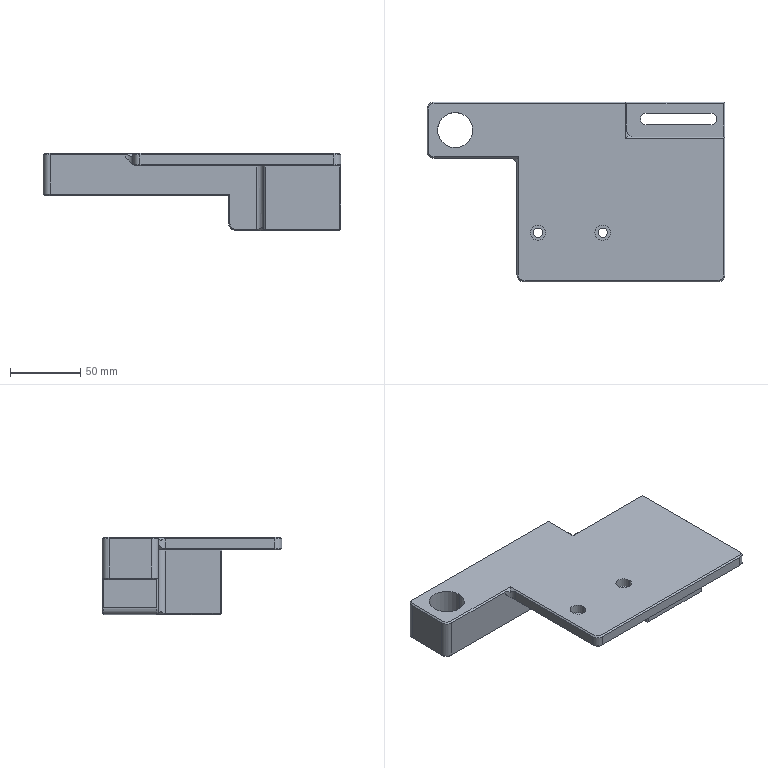NC program | NX | posted with a generic post | part box 212 x 128 x 55 mm
Lines 2820 to 4577 of 8014, first 1515 of 1754 lines:
(ZLEVEL_PROFILE_COPY_COPY_COPY_COPY , TOOL : D17R0.8)
N5632 T19 M6
N5634 G54
N5636 G17 G0 G90 X-28.227 Y13.355 S2000 M3
N5638 G43 Z30. H19
N5640 Z-0.3
N5642 G94 G1 X-29.568 Y15.677 F1000.
N5644 G3 X-31.04 Y16.527 R1.7
N5646 G1 X-43.527 F2000.
N5648 Y3.063
N5650 G3 X-42.677 Y1.59 R1.7
N5652 G1 X-40.127 Y0.118
N5654 G0 X-26.374 Y13.496 Z-0.6
N5656 G1 X-27.97 Y15.643 F1000.
N5658 G3 X-29.53 Y16.318 R1.7
N5660 G2 X-31. Y16.227 R13.652 F2000.
N5662 G1 X-43.227
N5664 Y0.892
N5666 G3 X-42.377 Y-0.58 R1.7
N5668 G1 X-39.827 Y-2.053
N5670 G0 X-26.137 Y13.28 Z-0.9
N5672 G1 X-27.774 Y15.404 F1000.
N5674 G3 X-29.346 Y16.05 R1.7
N5676 G2 X-31. Y15.927 R14.084 F2000.
N5678 G1 X-42.927
N5680 Y0.64
N5682 G3 X-42.077 Y-0.832 R1.7
N5684 G1 X-39.527 Y-2.304
N5686 G0 X-26.071 Y13.026 Z-1.2
N5688 G1 X-27.73 Y15.138 F1000.
N5690 G3 X-29.308 Y15.771 R1.7
N5692 G2 X-31.012 Y15.629 R14.424 F2000.
N5694 G1 X-42.629
N5696 Y0.569
N5698 G3 X-41.779 Y-0.904 R1.7
N5700 G1 X-39.229 Y-2.376
N5702 G0 X-26.037 Y12.748 Z-1.5
N5704 G1 X-27.588 Y14.865 F1000.
N5706 G3 X-29.144 Y15.549 R1.7
N5708 G2 X-30.099 Y15.488 R10.701 F2000.
N5710 G1 X-30.957 Y15.471
N5712 X-31.011 Y15.451
N5714 X-42.451
N5716 Y1.17
N5718 G3 X-41.601 Y-0.302 R1.7
N5720 G1 X-39.051 Y-1.774
N5722 G0 X-26.066 Y12.553 Z-1.8
N5724 G1 X-27.579 Y14.73 F1000.
N5726 G3 X-29.117 Y15.455 R1.7
N5728 G2 X-30.422 Y15.4 R15.644 F2000.
N5730 G1 X-42.4
N5732 Y1.03
N5734 G3 X-41.55 Y-0.442 R1.7
N5736 G1 X-39. Y-1.914
N5738 G0 X-25.877 Y12.452 Z-2.1
N5740 G1 X-27.297 Y14.641 F1000.
N5742 G3 X-28.811 Y15.413 R1.7
N5744 G2 X-29.33 Y15.4 R10.016 F2000.
N5746 G1 X-42.4
N5748 Y0.104
N5750 G3 X-41.55 Y-1.369 R1.7
N5752 G1 X-39. Y-2.841
N5754 G0 X-25.403 Y12.466 Z-2.4
N5756 G1 X-26.824 Y14.645 F1000.
N5758 G3 X-28.34 Y15.414 R1.7
N5760 G2 X-28.864 Y15.4 R9.678 F2000.
N5762 G1 X-42.4
N5764 Y0.011
N5766 G3 X-41.55 Y-1.461 R1.7
N5768 G1 X-39. Y-2.933
N5770 G0 X-25.124 Y12.447 Z-2.7
N5772 G1 X-26.527 Y14.632 F1000.
N5774 G3 X-28.038 Y15.411 R1.7
N5776 G2 X-28.475 Y15.4 R9.485 F2000.
N5778 G1 X-42.4
N5780 Y-0.04
N5782 G3 X-41.55 Y-1.512 R1.7
N5784 G1 X-39. Y-2.985
N5786 G0 X-24.937 Y12.419 Z-3.
N5788 G1 X-26.31 Y14.61 F1000.
N5790 G3 X-27.812 Y15.406 R1.7
N5792 G2 X-28.141 Y15.4 R9.072 F2000.
N5794 G1 X-42.4
N5796 Y-0.075
N5798 G3 X-41.55 Y-1.547 R1.7
N5800 G1 X-39. Y-3.019
N5802 G0 X-24.822 Y12.385 Z-3.3
N5804 G1 X-26.168 Y14.589 F1000.
N5806 G3 X-27.661 Y15.403 R1.7
N5808 G2 X-27.879 Y15.4 R8.949 F2000.
N5810 G1 X-42.4
N5812 Y-0.097
N5814 G3 X-41.55 Y-1.569 R1.7
N5816 G1 X-39. Y-3.041
N5818 G0 X-24.674 Y12.375 Z-3.6
N5820 G1 X-26.013 Y14.584 F1000.
N5822 G3 X-27.503 Y15.402 R1.7
N5824 G1 X-27.659 Y15.4 F2000.
N5826 X-42.4
N5828 Y-0.118
N5830 G3 X-41.55 Y-1.59 R1.7
N5832 G1 X-39. Y-3.062
N5834 G0 X-24.633 Y12.336 Z-3.9
N5836 G1 X-25.932 Y14.558 F1000.
N5838 G3 X-27.409 Y15.4 R1.7
N5840 G1 X-42.4 F2000.
N5842 Y-0.129
N5844 G3 X-41.55 Y-1.602 R1.7
N5846 G1 X-39. Y-3.074
N5848 G0 X-24.54 Y12.332 Z-4.2
N5850 G1 X-25.84 Y14.558 F1000.
N5852 G3 X-27.317 Y15.4 R1.7
N5854 G1 X-42.4 F2000.
N5856 Y-0.14
N5858 G3 X-41.55 Y-1.613 R1.7
N5860 G1 X-39. Y-3.085
N5862 G0 X-24.409 Y12.34 Z-4.5
N5864 G1 X-25.715 Y14.562 F1000.
N5866 G3 X-27.194 Y15.4 R1.7
N5868 G1 X-42.4 F2000.
N5870 Y-0.154
N5872 G3 X-41.55 Y-1.626 R1.7
N5874 G1 X-39. Y-3.099
N5876 G0 X-24.384 Y12.327 Z-4.8
N5878 G1 X-25.682 Y14.556 F1000.
N5880 G3 X-27.158 Y15.4 R1.7
N5882 G1 X-42.4 F2000.
N5884 Y-0.158
N5886 G3 X-41.55 Y-1.63 R1.7
N5888 G1 X-39. Y-3.103
N5890 G0 X-24.358 Y12.311 Z-5.1
N5892 G1 X-25.651 Y14.55 F1000.
N5894 G3 X-27.123 Y15.4 R1.7
N5896 G1 X-42.4 F2000.
N5898 Y-0.162
N5900 G3 X-41.55 Y-1.634 R1.7
N5902 G1 X-39. Y-3.106
N5904 G0 X-24.286 Y12.317 Z-5.4
N5906 G1 X-25.576 Y14.55 F1000.
N5908 G3 X-27.048 Y15.4 R1.7
N5910 G1 X-42.4 F2000.
N5912 Y-0.192
N5914 G3 X-41.55 Y-1.664 R1.7
N5916 G1 X-39. Y-3.136
N5918 G0 X-24.272 Y12.315 Z-5.7
N5920 G1 X-25.563 Y14.55 F1000.
N5922 G3 X-27.035 Y15.4 R1.7
N5924 G1 X-42.4 F2000.
N5926 Y-0.192
N5928 G3 X-41.55 Y-1.664 R1.7
N5930 G1 X-39. Y-3.136
N5932 G0 X-24.3 Y12.308 Z-6.
N5934 G1 X-25.595 Y14.55 F1000.
N5936 G3 X-27.067 Y15.4 R1.7
N5938 G1 X-42.4 F2000.
N5940 Y-0.167
N5942 G3 X-41.55 Y-1.64 R1.7
N5944 G1 X-39. Y-3.112
N5946 G0 X-24.3 Y12.308 Z-6.3
N5948 G1 X-25.595 Y14.55 F1000.
N5950 G3 X-27.067 Y15.4 R1.7
N5952 G1 X-42.4 F2000.
N5954 Y-0.167
N5956 G3 X-41.55 Y-1.64 R1.7
N5958 G1 X-39. Y-3.112
N5960 G0 X-24.3 Y12.308 Z-6.6
N5962 G1 X-25.595 Y14.55 F1000.
N5964 G3 X-27.067 Y15.4 R1.7
N5966 G1 X-42.4 F2000.
N5968 Y-0.167
N5970 G3 X-41.55 Y-1.64 R1.7
N5972 G1 X-39. Y-3.112
N5974 G0 X-24.3 Y12.308 Z-6.9
N5976 G1 X-25.595 Y14.55 F1000.
N5978 G3 X-27.067 Y15.4 R1.7
N5980 G1 X-42.4 F2000.
N5982 Y-0.167
N5984 G3 X-41.55 Y-1.64 R1.7
N5986 G1 X-39. Y-3.112
N5988 G0 X-24.3 Y12.308 Z-7.2
N5990 G1 X-25.595 Y14.55 F1000.
N5992 G3 X-27.067 Y15.4 R1.7
N5994 G1 X-42.4 F2000.
N5996 Y-0.167
N5998 G3 X-41.55 Y-1.64 R1.7
N6000 G1 X-39. Y-3.112
N6002 G0 X-24.3 Y12.308 Z-7.5
N6004 G1 X-25.595 Y14.55 F1000.
N6006 G3 X-27.067 Y15.4 R1.7
N6008 G1 X-42.4 F2000.
N6010 Y-0.167
N6012 G3 X-41.55 Y-1.64 R1.7
N6014 G1 X-39. Y-3.112
N6016 G0 X-24.3 Y12.308 Z-7.8
N6018 G1 X-25.595 Y14.55 F1000.
N6020 G3 X-27.067 Y15.4 R1.7
N6022 G1 X-42.4 F2000.
N6024 Y-0.167
N6026 G3 X-41.55 Y-1.64 R1.7
N6028 G1 X-39. Y-3.112
N6030 G0 X-24.3 Y12.308 Z-8.1
N6032 G1 X-25.595 Y14.55 F1000.
N6034 G3 X-27.067 Y15.4 R1.7
N6036 G1 X-42.4 F2000.
N6038 Y-0.167
N6040 G3 X-41.55 Y-1.64 R1.7
N6042 G1 X-39. Y-3.112
N6044 G0 X-24.3 Y12.308 Z-8.4
N6046 G1 X-25.595 Y14.55 F1000.
N6048 G3 X-27.067 Y15.4 R1.7
N6050 G1 X-42.4 F2000.
N6052 Y-0.167
N6054 G3 X-41.55 Y-1.64 R1.7
N6056 G1 X-39. Y-3.112
N6058 G0 X-24.3 Y12.308 Z-8.7
N6060 G1 X-25.595 Y14.55 F1000.
N6062 G3 X-27.067 Y15.4 R1.7
N6064 G1 X-42.4 F2000.
N6066 Y-0.167
N6068 G3 X-41.55 Y-1.64 R1.7
N6070 G1 X-39. Y-3.112
N6072 G0 X-24.3 Y12.308 Z-9.
N6074 G1 X-25.595 Y14.55 F1000.
N6076 G3 X-27.067 Y15.4 R1.7
N6078 G1 X-42.4 F2000.
N6080 Y-0.167
N6082 G3 X-41.55 Y-1.64 R1.7
N6084 G1 X-39. Y-3.112
N6086 G0 X-24.3 Y12.308 Z-9.3
N6088 G1 X-25.595 Y14.55 F1000.
N6090 G3 X-27.067 Y15.4 R1.7
N6092 G1 X-42.4 F2000.
N6094 Y-0.167
N6096 G3 X-41.55 Y-1.64 R1.7
N6098 G1 X-39. Y-3.112
N6100 G0 X-24.3 Y12.308 Z-9.6
N6102 G1 X-25.595 Y14.55 F1000.
N6104 G3 X-27.067 Y15.4 R1.7
N6106 G1 X-42.4 F2000.
N6108 Y-0.167
N6110 G3 X-41.55 Y-1.64 R1.7
N6112 G1 X-39. Y-3.112
N6114 G0 X-24.3 Y12.308 Z-9.9
N6116 G1 X-25.595 Y14.55 F1000.
N6118 G3 X-27.067 Y15.4 R1.7
N6120 G1 X-42.4 F2000.
N6122 Y-0.167
N6124 G3 X-41.55 Y-1.64 R1.7
N6126 G1 X-39. Y-3.112
N6128 G0 X-24.3 Y12.308 Z-10.2
N6130 G1 X-25.595 Y14.55 F1000.
N6132 G3 X-27.067 Y15.4 R1.7
N6134 G1 X-42.4 F2000.
N6136 Y-0.167
N6138 G3 X-41.55 Y-1.64 R1.7
N6140 G1 X-39. Y-3.112
N6142 G0 X-24.3 Y12.308 Z-10.5
N6144 G1 X-25.595 Y14.55 F1000.
N6146 G3 X-27.067 Y15.4 R1.7
N6148 G1 X-42.4 F2000.
N6150 Y-0.167
N6152 G3 X-41.55 Y-1.64 R1.7
N6154 G1 X-39. Y-3.112
N6156 G0 X-24.3 Y12.308 Z-10.8
N6158 G1 X-25.595 Y14.55 F1000.
N6160 G3 X-27.067 Y15.4 R1.7
N6162 G1 X-42.4 F2000.
N6164 Y-0.167
N6166 G3 X-41.55 Y-1.64 R1.7
N6168 G1 X-39. Y-3.112
N6170 G0 X-24.3 Y12.308 Z-11.1
N6172 G1 X-25.595 Y14.55 F1000.
N6174 G3 X-27.067 Y15.4 R1.7
N6176 G1 X-42.4 F2000.
N6178 Y-0.167
N6180 G3 X-41.55 Y-1.64 R1.7
N6182 G1 X-39. Y-3.112
N6184 G0 X-24.3 Y12.308 Z-11.4
N6186 G1 X-25.595 Y14.55 F1000.
N6188 G3 X-27.067 Y15.4 R1.7
N6190 G1 X-42.4 F2000.
N6192 Y-0.167
N6194 G3 X-41.55 Y-1.64 R1.7
N6196 G1 X-39. Y-3.112
N6198 G0 X-24.3 Y12.308 Z-11.7
N6200 G1 X-25.595 Y14.55 F1000.
N6202 G3 X-27.067 Y15.4 R1.7
N6204 G1 X-42.4 F2000.
N6206 Y-0.167
N6208 G3 X-41.55 Y-1.64 R1.7
N6210 G1 X-39. Y-3.112
N6212 G0 X-24.3 Y12.308 Z-12.
N6214 G1 X-25.595 Y14.55 F1000.
N6216 G3 X-27.067 Y15.4 R1.7
N6218 G1 X-42.4 F2000.
N6220 Y-0.167
N6222 G3 X-41.55 Y-1.64 R1.7
N6224 G1 X-39. Y-3.112
N6226 G0 X-24.3 Y12.308 Z-12.3
N6228 G1 X-25.595 Y14.55 F1000.
N6230 G3 X-27.067 Y15.4 R1.7
N6232 G1 X-42.4 F2000.
N6234 Y-0.167
N6236 G3 X-41.55 Y-1.64 R1.7
N6238 G1 X-39. Y-3.112
N6240 G0 X-24.3 Y12.308 Z-12.6
N6242 G1 X-25.595 Y14.55 F1000.
N6244 G3 X-27.067 Y15.4 R1.7
N6246 G1 X-42.4 F2000.
N6248 Y-0.167
N6250 G3 X-41.55 Y-1.64 R1.7
N6252 G1 X-39. Y-3.112
N6254 G0 X-24.3 Y12.308 Z-12.9
N6256 G1 X-25.595 Y14.55 F1000.
N6258 G3 X-27.067 Y15.4 R1.7
N6260 G1 X-42.4 F2000.
N6262 Y-0.167
N6264 G3 X-41.55 Y-1.64 R1.7
N6266 G1 X-39. Y-3.112
N6268 G0 X-24.3 Y12.308 Z-13.2
N6270 G1 X-25.595 Y14.55 F1000.
N6272 G3 X-27.067 Y15.4 R1.7
N6274 G1 X-42.4 F2000.
N6276 Y-0.167
N6278 G3 X-41.55 Y-1.64 R1.7
N6280 G1 X-39. Y-3.112
N6282 G0 X-24.3 Y12.308 Z-13.5
N6284 G1 X-25.595 Y14.55 F1000.
N6286 G3 X-27.067 Y15.4 R1.7
N6288 G1 X-42.4 F2000.
N6290 Y-0.167
N6292 G3 X-41.55 Y-1.64 R1.7
N6294 G1 X-39. Y-3.112
N6296 G0 X-24.3 Y12.308 Z-13.8
N6298 G1 X-25.595 Y14.55 F1000.
N6300 G3 X-27.067 Y15.4 R1.7
N6302 G1 X-42.4 F2000.
N6304 Y-0.167
N6306 G3 X-41.55 Y-1.64 R1.7
N6308 G1 X-39. Y-3.112
N6310 G0 X-24.3 Y12.308 Z-14.1
N6312 G1 X-25.595 Y14.55 F1000.
N6314 G3 X-27.067 Y15.4 R1.7
N6316 G1 X-42.4 F2000.
N6318 Y-0.167
N6320 G3 X-41.55 Y-1.64 R1.7
N6322 G1 X-39. Y-3.112
N6324 G0 X-24.3 Y12.308 Z-14.4
N6326 G1 X-25.595 Y14.55 F1000.
N6328 G3 X-27.067 Y15.4 R1.7
N6330 G1 X-42.4 F2000.
N6332 Y-0.167
N6334 G3 X-41.55 Y-1.64 R1.7
N6336 G1 X-39. Y-3.112
N6338 G0 X-24.3 Y12.308 Z-14.7
N6340 G1 X-25.595 Y14.55 F1000.
N6342 G3 X-27.067 Y15.4 R1.7
N6344 G1 X-42.4 F2000.
N6346 Y-0.167
N6348 G3 X-41.55 Y-1.64 R1.7
N6350 G1 X-39. Y-3.112
N6352 G0 X-24.3 Y12.308 Z-15.
N6354 G1 X-25.595 Y14.55 F1000.
N6356 G3 X-27.067 Y15.4 R1.7
N6358 G1 X-42.4 F2000.
N6360 Y-0.167
N6362 G3 X-41.55 Y-1.64 R1.7
N6364 G1 X-39. Y-3.112
N6366 G0 X-24.3 Y12.308 Z-15.3
N6368 G1 X-25.595 Y14.55 F1000.
N6370 G3 X-27.067 Y15.4 R1.7
N6372 G1 X-42.4 F2000.
N6374 Y-0.167
N6376 G3 X-41.55 Y-1.64 R1.7
N6378 G1 X-39. Y-3.112
N6380 G0 X-24.3 Y12.308 Z-15.6
N6382 G1 X-25.595 Y14.55 F1000.
N6384 G3 X-27.067 Y15.4 R1.7
N6386 G1 X-42.4 F2000.
N6388 Y-0.167
N6390 G3 X-41.55 Y-1.64 R1.7
N6392 G1 X-39. Y-3.112
N6394 G0 X-24.3 Y12.308 Z-15.9
N6396 G1 X-25.595 Y14.55 F1000.
N6398 G3 X-27.067 Y15.4 R1.7
N6400 G1 X-42.4 F2000.
N6402 Y-0.167
N6404 G3 X-41.55 Y-1.64 R1.7
N6406 G1 X-39. Y-3.112
N6408 G0 X-24.3 Y12.308 Z-16.2
N6410 G1 X-25.595 Y14.55 F1000.
N6412 G3 X-27.067 Y15.4 R1.7
N6414 G1 X-42.4 F2000.
N6416 Y-0.167
N6418 G3 X-41.55 Y-1.64 R1.7
N6420 G1 X-39. Y-3.112
N6422 G0 X-24.3 Y12.308 Z-16.5
N6424 G1 X-25.595 Y14.55 F1000.
N6426 G3 X-27.067 Y15.4 R1.7
N6428 G1 X-42.4 F2000.
N6430 Y-0.167
N6432 G3 X-41.55 Y-1.64 R1.7
N6434 G1 X-39. Y-3.112
N6436 G0 X-24.3 Y12.308 Z-16.8
N6438 G1 X-25.595 Y14.55 F1000.
N6440 G3 X-27.067 Y15.4 R1.7
N6442 G1 X-42.4 F2000.
N6444 Y-0.167
N6446 G3 X-41.55 Y-1.64 R1.7
N6448 G1 X-39. Y-3.112
N6450 G0 X-24.3 Y12.308 Z-17.1
N6452 G1 X-25.595 Y14.55 F1000.
N6454 G3 X-27.067 Y15.4 R1.7
N6456 G1 X-42.4 F2000.
N6458 Y-0.167
N6460 G3 X-41.55 Y-1.64 R1.7
N6462 G1 X-39. Y-3.112
N6464 G0 X-24.3 Y12.308 Z-17.4
N6466 G1 X-25.595 Y14.55 F1000.
N6468 G3 X-27.067 Y15.4 R1.7
N6470 G1 X-42.4 F2000.
N6472 Y-0.167
N6474 G3 X-41.55 Y-1.64 R1.7
N6476 G1 X-39. Y-3.112
N6478 G0 X-24.3 Y12.308 Z-17.7
N6480 G1 X-25.595 Y14.55 F1000.
N6482 G3 X-27.067 Y15.4 R1.7
N6484 G1 X-42.4 F2000.
N6486 Y-0.167
N6488 G3 X-41.55 Y-1.64 R1.7
N6490 G1 X-39. Y-3.112
N6492 G0 X-24.3 Y12.308 Z-18.
N6494 G1 X-25.595 Y14.55 F1000.
N6496 G3 X-27.067 Y15.4 R1.7
N6498 G1 X-42.4 F2000.
N6500 Y-0.167
N6502 G3 X-41.55 Y-1.64 R1.7
N6504 G1 X-39. Y-3.112
N6506 G0 X-24.3 Y12.308 Z-18.3
N6508 G1 X-25.595 Y14.55 F1000.
N6510 G3 X-27.067 Y15.4 R1.7
N6512 G1 X-42.4 F2000.
N6514 Y-0.167
N6516 G3 X-41.55 Y-1.64 R1.7
N6518 G1 X-39. Y-3.112
N6520 G0 X-24.3 Y12.308 Z-18.6
N6522 G1 X-25.595 Y14.55 F1000.
N6524 G3 X-27.067 Y15.4 R1.7
N6526 G1 X-42.4 F2000.
N6528 Y-0.167
N6530 G3 X-41.55 Y-1.64 R1.7
N6532 G1 X-39. Y-3.112
N6534 G0 X-24.3 Y12.308 Z-18.9
N6536 G1 X-25.595 Y14.55 F1000.
N6538 G3 X-27.067 Y15.4 R1.7
N6540 G1 X-42.4 F2000.
N6542 Y-0.167
N6544 G3 X-41.55 Y-1.64 R1.7
N6546 G1 X-39. Y-3.112
N6548 G0 X-24.3 Y12.308 Z-19.2
N6550 G1 X-25.595 Y14.55 F1000.
N6552 G3 X-27.067 Y15.4 R1.7
N6554 G1 X-42.4 F2000.
N6556 Y-0.167
N6558 G3 X-41.55 Y-1.64 R1.7
N6560 G1 X-39. Y-3.112
N6562 G0 X-24.3 Y12.308 Z-19.5
N6564 G1 X-25.595 Y14.55 F1000.
N6566 G3 X-27.067 Y15.4 R1.7
N6568 G1 X-42.4 F2000.
N6570 Y-0.167
N6572 G3 X-41.55 Y-1.64 R1.7
N6574 G1 X-39. Y-3.112
N6576 G0 X-24.3 Y12.308 Z-19.8
N6578 G1 X-25.595 Y14.55 F1000.
N6580 G3 X-27.067 Y15.4 R1.7
N6582 G1 X-42.4 F2000.
N6584 Y-0.167
N6586 G3 X-41.55 Y-1.64 R1.7
N6588 G1 X-39. Y-3.112
N6590 G0 X-24.3 Y12.308 Z-20.1
N6592 G1 X-25.595 Y14.55 F1000.
N6594 G3 X-27.067 Y15.4 R1.7
N6596 G1 X-42.4 F2000.
N6598 Y-0.167
N6600 G3 X-41.55 Y-1.64 R1.7
N6602 G1 X-39. Y-3.112
N6604 G0 X-24.3 Y12.308 Z-20.4
N6606 G1 X-25.595 Y14.55 F1000.
N6608 G3 X-27.067 Y15.4 R1.7
N6610 G1 X-42.4 F2000.
N6612 Y-0.167
N6614 G3 X-41.55 Y-1.64 R1.7
N6616 G1 X-39. Y-3.112
N6618 G0 X-24.3 Y12.308 Z-20.7
N6620 G1 X-25.595 Y14.55 F1000.
N6622 G3 X-27.067 Y15.4 R1.7
N6624 G1 X-42.4 F2000.
N6626 Y-0.167
N6628 G3 X-41.55 Y-1.64 R1.7
N6630 G1 X-39. Y-3.112
N6632 G0 X-24.3 Y12.308 Z-21.
N6634 G1 X-25.595 Y14.55 F1000.
N6636 G3 X-27.067 Y15.4 R1.7
N6638 G1 X-42.4 F2000.
N6640 Y-0.167
N6642 G3 X-41.55 Y-1.64 R1.7
N6644 G1 X-39. Y-3.112
N6646 G0 X-24.3 Y12.308 Z-21.3
N6648 G1 X-25.595 Y14.55 F1000.
N6650 G3 X-27.067 Y15.4 R1.7
N6652 G1 X-42.4 F2000.
N6654 Y-0.167
N6656 G3 X-41.55 Y-1.64 R1.7
N6658 G1 X-39. Y-3.112
N6660 G0 X-24.3 Y12.308 Z-21.6
N6662 G1 X-25.595 Y14.55 F1000.
N6664 G3 X-27.067 Y15.4 R1.7
N6666 G1 X-42.4 F2000.
N6668 Y-0.167
N6670 G3 X-41.55 Y-1.64 R1.7
N6672 G1 X-39. Y-3.112
N6674 G0 X-24.3 Y12.308 Z-21.9
N6676 G1 X-25.595 Y14.55 F1000.
N6678 G3 X-27.067 Y15.4 R1.7
N6680 G1 X-42.4 F2000.
N6682 Y-0.167
N6684 G3 X-41.55 Y-1.64 R1.7
N6686 G1 X-39. Y-3.112
N6688 G0 X-24.3 Y12.308 Z-22.2
N6690 G1 X-25.595 Y14.55 F1000.
N6692 G3 X-27.067 Y15.4 R1.7
N6694 G1 X-42.4 F2000.
N6696 Y-0.167
N6698 G3 X-41.55 Y-1.64 R1.7
N6700 G1 X-39. Y-3.112
N6702 G0 X-24.3 Y12.308 Z-22.5
N6704 G1 X-25.595 Y14.55 F1000.
N6706 G3 X-27.067 Y15.4 R1.7
N6708 G1 X-42.4 F2000.
N6710 Y-0.167
N6712 G3 X-41.55 Y-1.64 R1.7
N6714 G1 X-39. Y-3.112
N6716 G0 X-24.3 Y12.308 Z-22.8
N6718 G1 X-25.595 Y14.55 F1000.
N6720 G3 X-27.067 Y15.4 R1.7
N6722 G1 X-42.4 F2000.
N6724 Y-0.167
N6726 G3 X-41.55 Y-1.64 R1.7
N6728 G1 X-39. Y-3.112
N6730 G0 X-24.3 Y12.308 Z-23.1
N6732 G1 X-25.595 Y14.55 F1000.
N6734 G3 X-27.067 Y15.4 R1.7
N6736 G1 X-42.4 F2000.
N6738 Y-0.167
N6740 G3 X-41.55 Y-1.64 R1.7
N6742 G1 X-39. Y-3.112
N6744 G0 X-24.3 Y12.308 Z-23.4
N6746 G1 X-25.595 Y14.55 F1000.
N6748 G3 X-27.067 Y15.4 R1.7
N6750 G1 X-42.4 F2000.
N6752 Y-0.167
N6754 G3 X-41.55 Y-1.64 R1.7
N6756 G1 X-39. Y-3.112
N6758 G0 X-24.3 Y12.308 Z-23.7
N6760 G1 X-25.595 Y14.55 F1000.
N6762 G3 X-27.067 Y15.4 R1.7
N6764 G1 X-42.4 F2000.
N6766 Y-0.167
N6768 G3 X-41.55 Y-1.64 R1.7
N6770 G1 X-39. Y-3.112
N6772 G0 X-24.3 Y12.308 Z-24.
N6774 G1 X-25.595 Y14.55 F1000.
N6776 G3 X-27.067 Y15.4 R1.7
N6778 G1 X-42.4 F2000.
N6780 Y-0.167
N6782 G3 X-41.55 Y-1.64 R1.7
N6784 G1 X-39. Y-3.112
N6786 G0 X-24.3 Y12.308 Z-24.3
N6788 G1 X-25.595 Y14.55 F1000.
N6790 G3 X-27.067 Y15.4 R1.7
N6792 G1 X-42.4 F2000.
N6794 Y-0.167
N6796 G3 X-41.55 Y-1.64 R1.7
N6798 G1 X-39. Y-3.112
N6800 G0 X-24.3 Y12.308 Z-24.6
N6802 G1 X-25.595 Y14.55 F1000.
N6804 G3 X-27.067 Y15.4 R1.7
N6806 G1 X-42.4 F2000.
N6808 Y-0.167
N6810 G3 X-41.55 Y-1.64 R1.7
N6812 G1 X-39. Y-3.112
N6814 G0 X-24.3 Y12.308 Z-24.9
N6816 G1 X-25.595 Y14.55 F1000.
N6818 G3 X-27.067 Y15.4 R1.7
N6820 G1 X-42.4 F2000.
N6822 Y-0.167
N6824 G3 X-41.55 Y-1.64 R1.7
N6826 G1 X-39. Y-3.112
N6828 G0 X-24.3 Y12.308 Z-25.2
N6830 G1 X-25.595 Y14.55 F1000.
N6832 G3 X-27.067 Y15.4 R1.7
N6834 G1 X-42.4 F2000.
N6836 Y-0.167
N6838 G3 X-41.55 Y-1.64 R1.7
N6840 G1 X-39. Y-3.112
N6842 G0 X-24.3 Y12.308 Z-25.5
N6844 G1 X-25.595 Y14.55 F1000.
N6846 G3 X-27.067 Y15.4 R1.7
N6848 G1 X-42.4 F2000.
N6850 Y-0.167
N6852 G3 X-41.55 Y-1.64 R1.7
N6854 G1 X-39. Y-3.112
N6856 G0 X-24.3 Y12.308 Z-25.8
N6858 G1 X-25.595 Y14.55 F1000.
N6860 G3 X-27.067 Y15.4 R1.7
N6862 G1 X-42.4 F2000.
N6864 Y-0.167
N6866 G3 X-41.55 Y-1.64 R1.7
N6868 G1 X-39. Y-3.112
N6870 G0 X-24.3 Y12.308 Z-26.1
N6872 G1 X-25.595 Y14.55 F1000.
N6874 G3 X-27.067 Y15.4 R1.7
N6876 G1 X-42.4 F2000.
N6878 Y-0.167
N6880 G3 X-41.55 Y-1.64 R1.7
N6882 G1 X-39. Y-3.112
N6884 G0 X-24.177 Y12.094 Z-26.4
N6886 G1 X-25.595 Y14.55 F1000.
N6888 G3 X-27.067 Y15.4 R1.7
N6890 G1 X-42.4 F2000.
N6892 Y-0.167
N6894 G3 X-41.55 Y-1.64 R1.7
N6896 G1 X-39. Y-3.112
N6898 G0 X-24.126 Y12.006 Z-26.7
N6900 G1 X-25.595 Y14.55 F1000.
N6902 G3 X-27.067 Y15.4 R1.7
N6904 G1 X-42.4 F2000.
N6906 Y-0.167
N6908 G3 X-41.55 Y-1.64 R1.7
N6910 G1 X-39. Y-3.112
N6912 G0 X-23.9 Y12. Z-27.
N6914 G1 X-25.373 Y14.55 F1000.
N6916 G3 X-26.845 Y15.4 R1.7
N6918 G1 X-42.4 F2000.
N6920 Y-0.188
N6922 G3 X-41.55 Y-1.661 R1.7
N6924 G1 X-39. Y-3.133
N6926 G0 X-23.9 Y12. Z-27.3
N6928 G1 X-25.372 Y14.55 F1000.
N6930 G3 X-26.844 Y15.4 R1.7
N6932 G1 X-42.4 F2000.
N6934 Y-0.189
N6936 G3 X-41.55 Y-1.661 R1.7
N6938 G1 X-39. Y-3.133
N6940 G0 X-23.899 Y12. Z-27.6
N6942 G1 X-25.371 Y14.55 F1000.
N6944 G3 X-26.843 Y15.4 R1.7
N6946 G1 X-42.4 F2000.
N6948 Y-0.189
N6950 G3 X-41.55 Y-1.661 R1.7
N6952 G1 X-39. Y-3.133
N6954 G0 X-23.898 Y12. Z-27.9
N6956 G1 X-25.37 Y14.55 F1000.
N6958 G3 X-26.843 Y15.4 R1.7
N6960 G1 X-42.4 F2000.
N6962 Y-0.189
N6964 G3 X-41.55 Y-1.661 R1.7
N6966 G1 X-39. Y-3.133
N6968 G0 X-23.897 Y12. Z-28.2
N6970 G1 X-25.37 Y14.55 F1000.
N6972 G3 X-26.842 Y15.4 R1.7
N6974 G1 X-42.4 F2000.
N6976 Y-0.189
N6978 G3 X-41.55 Y-1.661 R1.7
N6980 G1 X-39. Y-3.133
N6982 G0 X-23.897 Y12. Z-28.5
N6984 G1 X-25.369 Y14.55 F1000.
N6986 G3 X-26.841 Y15.4 R1.7
N6988 G1 X-42.4 F2000.
N6990 Y-0.189
N6992 G3 X-41.55 Y-1.661 R1.7
N6994 G1 X-39. Y-3.133
N6996 G0 X-23.896 Y12. Z-28.8
N6998 G1 X-25.368 Y14.55 F1000.
N7000 G3 X-26.841 Y15.4 R1.7
N7002 G1 X-42.4 F2000.
N7004 Y-0.189
N7006 G3 X-41.55 Y-1.661 R1.7
N7008 G1 X-39. Y-3.133
N7010 G0 X-23.895 Y12. Z-29.1
N7012 G1 X-25.368 Y14.55 F1000.
N7014 G3 X-26.84 Y15.4 R1.7
N7016 G1 X-42.4 F2000.
N7018 Y-0.189
N7020 G3 X-41.55 Y-1.661 R1.7
N7022 G1 X-39. Y-3.133
N7024 G0 X-23.895 Y12. Z-29.4
N7026 G1 X-25.367 Y14.55 F1000.
N7028 G3 X-26.839 Y15.4 R1.7
N7030 G1 X-42.4 F2000.
N7032 Y-0.189
N7034 G3 X-41.55 Y-1.661 R1.7
N7036 G1 X-39. Y-3.133
N7038 G0 X-23.894 Y12. Z-29.7
N7040 G1 X-25.366 Y14.55 F1000.
N7042 G3 X-26.838 Y15.4 R1.7
N7044 G1 X-42.4 F2000.
N7046 Y-0.189
N7048 G3 X-41.55 Y-1.661 R1.7
N7050 G1 X-39. Y-3.134
N7052 G0 X-23.893 Y12. Z-30.
N7054 G1 X-25.365 Y14.55 F1000.
N7056 G3 X-26.838 Y15.4 R1.7
N7058 G1 X-42.4 F2000.
N7060 Y-0.189
N7062 G3 X-41.55 Y-1.661 R1.7
N7064 G1 X-39. Y-3.134
N7066 G0 X-23.892 Y12. Z-30.3
N7068 G1 X-25.365 Y14.55 F1000.
N7070 G3 X-26.837 Y15.4 R1.7
N7072 G1 X-42.4 F2000.
N7074 Y-0.189
N7076 G3 X-41.55 Y-1.661 R1.7
N7078 G1 X-39. Y-3.134
N7080 G0 X-23.892 Y12. Z-30.6
N7082 G1 X-25.364 Y14.55 F1000.
N7084 G3 X-26.836 Y15.4 R1.7
N7086 G1 X-42.4 F2000.
N7088 Y-0.189
N7090 G3 X-41.55 Y-1.661 R1.7
N7092 G1 X-39. Y-3.134
N7094 G0 X-23.891 Y12. Z-30.9
N7096 G1 X-25.363 Y14.55 F1000.
N7098 G3 X-26.835 Y15.4 R1.7
N7100 G1 X-42.4 F2000.
N7102 Y-0.189
N7104 G3 X-41.55 Y-1.662 R1.7
N7106 G1 X-39. Y-3.134
N7108 G0 X-23.89 Y12. Z-31.2
N7110 G1 X-25.362 Y14.55 F1000.
N7112 G3 X-26.835 Y15.4 R1.7
N7114 G1 X-42.4 F2000.
N7116 Y-0.189
N7118 G3 X-41.55 Y-1.662 R1.7
N7120 G1 X-39. Y-3.134
N7122 G0 X-23.889 Y12. Z-31.5
N7124 G1 X-25.362 Y14.55 F1000.
N7126 G3 X-26.834 Y15.4 R1.7
N7128 G1 X-42.4 F2000.
N7130 Y-0.189
N7132 G3 X-41.55 Y-1.662 R1.7
N7134 G1 X-39. Y-3.134
N7136 G0 X-23.889 Y12. Z-31.8
N7138 G1 X-25.361 Y14.55 F1000.
N7140 G3 X-26.833 Y15.4 R1.7
N7142 G1 X-42.4 F2000.
N7144 Y-0.189
N7146 G3 X-41.55 Y-1.662 R1.7
N7148 G1 X-39. Y-3.134
N7150 G0 X-23.888 Y12. Z-32.1
N7152 G1 X-25.36 Y14.55 F1000.
N7154 G3 X-26.832 Y15.4 R1.7
N7156 G1 X-42.4 F2000.
N7158 Y-0.19
N7160 G3 X-41.55 Y-1.662 R1.7
N7162 G1 X-39. Y-3.134
N7164 G0 X-23.887 Y12. Z-32.4
N7166 G1 X-25.359 Y14.55 F1000.
N7168 G3 X-26.832 Y15.4 R1.7
N7170 G1 X-42.4 F2000.
N7172 Y-0.19
N7174 G3 X-41.55 Y-1.662 R1.7
N7176 G1 X-39. Y-3.134
N7178 G0 X-23.886 Y12. Z-32.7
N7180 G1 X-25.359 Y14.55 F1000.
N7182 G3 X-26.831 Y15.4 R1.7
N7184 G1 X-42.4 F2000.
N7186 Y-0.19
N7188 G3 X-41.55 Y-1.662 R1.7
N7190 G1 X-39. Y-3.134
N7192 G0 X-23.886 Y12. Z-33.
N7194 G1 X-25.358 Y14.55 F1000.
N7196 G3 X-26.83 Y15.4 R1.7
N7198 G1 X-42.4 F2000.
N7200 Y-0.19
N7202 G3 X-41.55 Y-1.662 R1.7
N7204 G1 X-39. Y-3.134
N7206 G0 X-23.885 Y12. Z-33.3
N7208 G1 X-25.357 Y14.55 F1000.
N7210 G3 X-26.829 Y15.4 R1.7
N7212 G1 X-42.4 F2000.
N7214 Y-0.19
N7216 G3 X-41.55 Y-1.662 R1.7
N7218 G1 X-39. Y-3.134
N7220 G0 X-23.884 Y12. Z-33.6
N7222 G1 X-25.357 Y14.55 F1000.
N7224 G3 X-26.829 Y15.4 R1.7
N7226 G1 X-42.4 F2000.
N7228 Y-0.19
N7230 G3 X-41.55 Y-1.662 R1.7
N7232 G1 X-39. Y-3.134
N7234 G0 X-23.884 Y12. Z-33.9
N7236 G1 X-25.356 Y14.55 F1000.
N7238 G3 X-26.828 Y15.4 R1.7
N7240 G1 X-42.4 F2000.
N7242 Y-0.19
N7244 G3 X-41.55 Y-1.662 R1.7
N7246 G1 X-39. Y-3.134
N7248 G0 X-23.883 Y12. Z-34.2
N7250 G1 X-25.355 Y14.55 F1000.
N7252 G3 X-26.827 Y15.4 R1.7
N7254 G1 X-42.4 F2000.
N7256 Y-0.19
N7258 G3 X-41.55 Y-1.662 R1.7
N7260 G1 X-39. Y-3.134
N7262 G0 X-23.882 Y12. Z-34.5
N7264 G1 X-25.354 Y14.55 F1000.
N7266 G3 X-26.827 Y15.4 R1.7
N7268 G1 X-42.4 F2000.
N7270 Y-0.19
N7272 G3 X-41.55 Y-1.662 R1.7
N7274 G1 X-39. Y-3.135
N7276 G0 X-23.881 Y12. Z-34.8
N7278 G1 X-25.354 Y14.55 F1000.
N7280 G3 X-26.826 Y15.4 R1.7
N7282 G1 X-42.4 F2000.
N7284 Y-0.19
N7286 G3 X-41.55 Y-1.662 R1.7
N7288 G1 X-39. Y-3.135
N7290 G0 X-23.881 Y12. Z-35.1
N7292 G1 X-25.353 Y14.55 F1000.
N7294 G3 X-26.825 Y15.4 R1.7
N7296 G1 X-42.4 F2000.
N7298 Y-0.19
N7300 G3 X-41.55 Y-1.662 R1.7
N7302 G1 X-39. Y-3.135
N7304 G0 X-23.88 Y12. Z-35.4
N7306 G1 X-25.352 Y14.55 F1000.
N7308 G3 X-26.824 Y15.4 R1.7
N7310 G1 X-42.4 F2000.
N7312 Y-0.19
N7314 G3 X-41.55 Y-1.662 R1.7
N7316 G1 X-39. Y-3.135
N7318 G0 X-23.879 Y12. Z-35.7
N7320 G1 X-25.351 Y14.55 F1000.
N7322 G3 X-26.824 Y15.4 R1.7
N7324 G1 X-42.4 F2000.
N7326 Y-0.19
N7328 G3 X-41.55 Y-1.663 R1.7
N7330 G1 X-39. Y-3.135
N7332 G0 X-23.878 Y12. Z-36.
N7334 G1 X-25.351 Y14.55 F1000.
N7336 G3 X-26.823 Y15.4 R1.7
N7338 G1 X-42.4 F2000.
N7340 Y-0.19
N7342 G3 X-41.55 Y-1.663 R1.7
N7344 G1 X-39. Y-3.135
N7346 G0 X-23.878 Y12. Z-36.3
N7348 G1 X-25.35 Y14.55 F1000.
N7350 G3 X-26.822 Y15.4 R1.7
N7352 G1 X-42.4 F2000.
N7354 Y-0.19
N7356 G3 X-41.55 Y-1.663 R1.7
N7358 G1 X-39. Y-3.135
N7360 G0 X-23.877 Y12. Z-36.6
N7362 G1 X-25.349 Y14.55 F1000.
N7364 G3 X-26.821 Y15.4 R1.7
N7366 G1 X-42.4 F2000.
N7368 Y-0.19
N7370 G3 X-41.55 Y-1.663 R1.7
N7372 G1 X-39. Y-3.135
N7374 G0 X-23.876 Y12. Z-36.9
N7376 G1 X-25.348 Y14.55 F1000.
N7378 G3 X-26.821 Y15.4 R1.7
N7380 G1 X-42.4 F2000.
N7382 Y-0.191
N7384 G3 X-41.55 Y-1.663 R1.7
N7386 G1 X-39. Y-3.135
N7388 G0 X-23.875 Y12. Z-37.2
N7390 G1 X-25.348 Y14.55 F1000.
N7392 G3 X-26.82 Y15.4 R1.7
N7394 G1 X-42.4 F2000.
N7396 Y-0.191
N7398 G3 X-41.55 Y-1.663 R1.7
N7400 G1 X-39. Y-3.135
N7402 G0 X-23.875 Y12. Z-37.5
N7404 G1 X-25.347 Y14.55 F1000.
N7406 G3 X-26.819 Y15.4 R1.7
N7408 G1 X-42.4 F2000.
N7410 Y-0.191
N7412 G3 X-41.55 Y-1.663 R1.7
N7414 G1 X-39. Y-3.135
N7416 G0 X-23.874 Y12. Z-37.8
N7418 G1 X-25.346 Y14.55 F1000.
N7420 G3 X-26.818 Y15.4 R1.7
N7422 G1 X-42.4 F2000.
N7424 Y-0.191
N7426 G3 X-41.55 Y-1.663 R1.7
N7428 G1 X-39. Y-3.135
N7430 G0 X-23.873 Y12. Z-38.1
N7432 G1 X-25.345 Y14.55 F1000.
N7434 G3 X-26.818 Y15.4 R1.7
N7436 G1 X-42.4 F2000.
N7438 Y-0.191
N7440 G3 X-41.55 Y-1.663 R1.7
N7442 G1 X-39. Y-3.135
N7444 G0 X-23.872 Y12. Z-38.4
N7446 G1 X-25.345 Y14.55 F1000.
N7448 G3 X-26.817 Y15.4 R1.7
N7450 G1 X-42.4 F2000.
N7452 Y-0.191
N7454 G3 X-41.55 Y-1.663 R1.7
N7456 G1 X-39. Y-3.135
N7458 G0 X-23.872 Y12. Z-38.7
N7460 G1 X-25.344 Y14.55 F1000.
N7462 G3 X-26.816 Y15.4 R1.7
N7464 G1 X-42.4 F2000.
N7466 Y-0.191
N7468 G3 X-41.55 Y-1.663 R1.7
N7470 G1 X-39. Y-3.135
N7472 G0 X-23.871 Y12. Z-39.
N7474 G1 X-25.343 Y14.55 F1000.
N7476 G3 X-26.815 Y15.4 R1.7
N7478 G1 X-42.4 F2000.
N7480 Y-0.191
N7482 G3 X-41.55 Y-1.663 R1.7
N7484 G1 X-39. Y-3.135
N7486 G0 X-23.87 Y12. Z-39.3
N7488 G1 X-25.342 Y14.55 F1000.
N7490 G3 X-26.815 Y15.4 R1.7
N7492 G1 X-42.4 F2000.
N7494 Y-0.191
N7496 G3 X-41.55 Y-1.663 R1.7
N7498 G1 X-39. Y-3.136
N7500 G0 X-23.869 Y12. Z-39.6
N7502 G1 X-25.342 Y14.55 F1000.
N7504 G3 X-26.814 Y15.4 R1.7
N7506 G1 X-42.4 F2000.
N7508 Y-0.191
N7510 G3 X-41.55 Y-1.663 R1.7
N7512 G1 X-39. Y-3.136
N7514 G0 X-23.869 Y12. Z-39.9
N7516 G1 X-25.341 Y14.55 F1000.
N7518 G3 X-26.813 Y15.4 R1.7
N7520 G1 X-42.4 F2000.
N7522 Y-0.191
N7524 G3 X-41.55 Y-1.663 R1.7
N7526 G1 X-39. Y-3.136
N7528 G0 X-23.868 Y12. Z-40.2
N7530 G1 X-25.34 Y14.55 F1000.
N7532 G3 X-26.812 Y15.4 R1.7
N7534 G1 X-42.4 F2000.
N7536 Y-0.191
N7538 G3 X-41.55 Y-1.663 R1.7
N7540 G1 X-39. Y-3.136
N7542 G0 X-23.867 Y12. Z-40.5
N7544 G1 X-25.339 Y14.55 F1000.
N7546 G3 X-26.812 Y15.4 R1.7
N7548 G1 X-42.4 F2000.
N7550 Y-0.191
N7552 G3 X-41.55 Y-1.664 R1.7
N7554 G1 X-39. Y-3.136
N7556 G0 X-23.866 Y12. Z-40.8
N7558 G1 X-25.339 Y14.55 F1000.
N7560 G3 X-26.811 Y15.4 R1.7
N7562 G1 X-42.4 F2000.
N7564 Y-0.191
N7566 G3 X-41.55 Y-1.664 R1.7
N7568 G1 X-39. Y-3.136
N7570 G0 X-23.866 Y12. Z-41.1
N7572 G1 X-25.338 Y14.55 F1000.
N7574 G3 X-26.81 Y15.4 R1.7
N7576 G1 X-42.4 F2000.
N7578 Y-0.191
N7580 G3 X-41.55 Y-1.664 R1.7
N7582 G1 X-39. Y-3.136
N7584 G0 X-23.865 Y12. Z-41.4
N7586 G1 X-25.337 Y14.55 F1000.
N7588 G3 X-26.809 Y15.4 R1.7
N7590 G1 X-42.4 F2000.
N7592 Y-0.192
N7594 G3 X-41.55 Y-1.664 R1.7
N7596 G1 X-39. Y-3.136
N7598 G0 X-23.864 Y12. Z-41.7
N7600 G1 X-25.336 Y14.55 F1000.
N7602 G3 X-26.809 Y15.4 R1.7
N7604 G1 X-42.4 F2000.
N7606 Y-0.192
N7608 G3 X-41.55 Y-1.664 R1.7
N7610 G1 X-39. Y-3.136
N7612 G0 X-23.864 Y12. Z-42.
N7614 G1 X-25.336 Y14.55 F1000.
N7616 G3 X-26.808 Y15.4 R1.7
N7618 G1 X-42.4 F2000.
N7620 Y-0.192
N7622 G3 X-41.55 Y-1.664 R1.7
N7624 G1 X-39. Y-3.136
N7626 G0 X-23.864 Y12. Z-42.3
N7628 G1 X-25.336 Y14.55 F1000.
N7630 G3 X-26.808 Y15.4 R1.7
N7632 G1 X-42.4 F2000.
N7634 Y-0.192
N7636 G3 X-41.55 Y-1.664 R1.7
N7638 G1 X-39. Y-3.136
N7640 G0 X-23.864 Y12. Z-42.6
N7642 G1 X-25.336 Y14.55 F1000.
N7644 G3 X-26.808 Y15.4 R1.7
N7646 G1 X-42.4 F2000.
N7648 Y-0.192
N7650 G3 X-41.55 Y-1.664 R1.7
N7652 G1 X-39. Y-3.136
N7654 G0 X-23.864 Y12. Z-42.9
N7656 G1 X-25.336 Y14.55 F1000.
N7658 G3 X-26.808 Y15.4 R1.7
N7660 G1 X-42.4 F2000.
N7662 Y-0.192
N7664 G3 X-41.55 Y-1.664 R1.7
N7666 G1 X-39. Y-3.136
N7668 G0 X-23.864 Y12. Z-43.2
N7670 G1 X-25.336 Y14.55 F1000.
N7672 G3 X-26.808 Y15.4 R1.7
N7674 G1 X-42.4 F2000.
N7676 Y-0.192
N7678 G3 X-41.55 Y-1.664 R1.7
N7680 G1 X-39. Y-3.136
N7682 G0 X-23.864 Y12. Z-43.5
N7684 G1 X-25.336 Y14.55 F1000.
N7686 G3 X-26.808 Y15.4 R1.7
N7688 G1 X-42.4 F2000.
N7690 Y-0.192
N7692 G3 X-41.55 Y-1.664 R1.7
N7694 G1 X-39. Y-3.136
N7696 G0 X-23.864 Y12. Z-43.8
N7698 G1 X-25.336 Y14.55 F1000.
N7700 G3 X-26.808 Y15.4 R1.7
N7702 G1 X-42.4 F2000.
N7704 Y-0.192
N7706 G3 X-41.55 Y-1.664 R1.7
N7708 G1 X-39. Y-3.136
N7710 G0 X-23.864 Y12. Z-44.1
N7712 G1 X-25.336 Y14.55 F1000.
N7714 G3 X-26.808 Y15.4 R1.7
N7716 G1 X-42.4 F2000.
N7718 Y-0.192
N7720 G3 X-41.55 Y-1.664 R1.7
N7722 G1 X-39. Y-3.136
N7724 G0 X-23.864 Y12. Z-44.4
N7726 G1 X-25.336 Y14.55 F1000.
N7728 G3 X-26.808 Y15.4 R1.7
N7730 G1 X-42.4 F2000.
N7732 Y-0.192
N7734 G3 X-41.55 Y-1.664 R1.7
N7736 G1 X-39. Y-3.136
N7738 G0 X-23.864 Y12. Z-44.7
N7740 G1 X-25.336 Y14.55 F1000.
N7742 G3 X-26.808 Y15.4 R1.7
N7744 G1 X-42.4 F2000.
N7746 Y-0.192
N7748 G3 X-41.55 Y-1.664 R1.7
N7750 G1 X-39. Y-3.136
N7752 G0 X-23.864 Y12. Z-45.
N7754 G1 X-25.336 Y14.55 F1000.
N7756 G3 X-26.808 Y15.4 R1.7
N7758 G1 X-42.4 F2000.
N7760 Y-0.192
N7762 G3 X-41.55 Y-1.664 R1.7
N7764 G1 X-39. Y-3.136
N7766 G0 X-23.864 Y12. Z-45.3
N7768 G1 X-25.336 Y14.55 F1000.
N7770 G3 X-26.808 Y15.4 R1.7
N7772 G1 X-42.4 F2000.
N7774 Y-0.192
N7776 G3 X-41.55 Y-1.664 R1.7
N7778 G1 X-39. Y-3.136
N7780 G0 X-23.864 Y12. Z-45.6
N7782 G1 X-25.336 Y14.55 F1000.
N7784 G3 X-26.808 Y15.4 R1.7
N7786 G1 X-42.4 F2000.
N7788 Y-0.192
N7790 G3 X-41.55 Y-1.664 R1.7
N7792 G1 X-39. Y-3.136
N7794 G0 X-23.864 Y12. Z-45.9
N7796 G1 X-25.336 Y14.55 F1000.
N7798 G3 X-26.808 Y15.4 R1.7
N7800 G1 X-42.4 F2000.
N7802 Y-0.192
N7804 G3 X-41.55 Y-1.664 R1.7
N7806 G1 X-39. Y-3.136
N7808 G0 Z30.
N7810 X-18.926 Y12.927
N7812 Z-25.5
N7814 G1 X-20.398 Y15.477 F1000.
N7816 G3 X-21.87 Y16.327 R1.7
N7818 G1 X-23.116 F2000.
N7820 G2 X-23.818 Y16.01 R8.6
N7822 G3 X-24.871 Y14.676 R1.7
N7824 G1 X-25.242 Y12.13
N7826 G0 X-20.274 Y12.627 Z-25.8
N7828 G1 X-21.746 Y15.177 F1000.
N7830 G3 X-23.219 Y16.027 R1.7
N7832 G1 X-23.776 F2000.
N7834 G2 X-24.262 Y15.847 R8.6
N7836 G3 X-25.387 Y14.573 R1.7
N7838 G1 X-25.897 Y12.051
N7840 G0 Z30.
(ZLEVEL_PROFILE_COPY_1 , TOOL : D17R0.8)
N7842 X-16.855 Y80.327 S6000
N7844 Z2.994
N7846 G1 Z-0.006 F1000.
N7848 G3 X-23.211 Y72.351 R8.5
N7850 X-23.039 Y63. R97.923 F2500.
N7852 G1 Y25.
N7854 G3 X-23.218 Y15.648 R132.606
N7856 G1 X-23.151 Y15.649 Z-0.012
N7858 X-23.115 Y21.632
N7860 G2 X-22.927 Y25. R34.041
N7862 G1 Y63.
N7864 G2 X-23.132 Y66.127 R24.086
N7866 G1 X-23.136 Y72.35
N7868 X-23.097 Z-0.015
N7870 X-23.08 Z-0.019
N7872 X-23.06 Y65.591
N7874 X-23.016 Y64.427
N7876 X-22.832 Y63.
N7878 Y25.
N7880 G3 X-23.053 Y21.133 R39.093
N7882 G1 X-23.094 Y15.65
N7884 X-23.053 Z-0.023
N7886 X-23.034 Z-0.027
N7888 X-23.016 Y18.443
N7890 X-23.003 Y19.025
N7892 Y20.162
N7894 G2 X-22.744 Y25. R45.45
N7896 G1 Y63.
N7898 G3 X-22.933 Y64.427 R5.098
N7900 G1 X-22.987 Y65.591
N7902 X-23.018 Y72.35
N7904 X-22.949 Z-0.035
N7906 X-22.934 Y66.173
N7908 G3 X-22.66 Y63. R41.509
N7910 G1 Y25.
N7912 G3 X-22.931 Y19.607 R49.384
N7914 G1 X-22.932 Y19.025
N7916 X-22.948 Y18.443
N7918 X-22.969 Y15.65
N7920 X-22.904 Z-0.04
N7922 X-22.897 Z-0.045
N7924 X-22.873 Y18.443
N7926 X-22.853 Y19.025
N7928 X-22.848 Y20.332
N7930 G2 X-22.58 Y25. R43.215
N7932 G1 Y63.
N7934 X-22.819 Y65.591
N7936 X-22.851 Y66.173
N7938 X-22.874 Y72.35
N7940 X-22.788 Z-0.05
N7942 X-22.792 Z-0.055
N7944 X-22.788 Y66.755
N7946 X-22.501 Y63.
N7948 Y25.
N7950 G3 X-22.776 Y20.012 R55.118
N7952 G1 X-22.819 Y15.65
N7954 X-22.754 Z-0.061
N7956 X-22.733 Z-0.067
N7958 G2 X-22.424 Y25. R108.438
N7960 G1 Y63.
N7962 X-22.697 Y66.755
N7964 X-22.703 Y72.35
N7966 X-22.631 Z-0.073
N7968 X-22.607 Z-0.079
N7970 G3 X-22.348 Y63. R103.456
N7972 G1 Y25.
N7974 G3 X-22.642 Y15.65 R123.685
N7976 G1 X-22.589 Z-0.085
N7978 X-22.545 Z-0.092
N7980 X-22.52 Y18.443
N7982 X-22.498 Y19.025
N7984 G2 X-22.273 Y25. R48.746
N7986 G1 Y63.
N7988 X-22.461 Y65.591
N7990 X-22.487 Y66.173
N7992 X-22.519 Y72.35
N7994 X-22.477 Z-0.099
N7996 X-22.443 Z-0.106
N7998 X-22.411 Y66.173
N8000 X-22.387 Y65.591
N8002 X-22.194 Y63.
N8004 Y25.
N8006 G3 X-22.437 Y20.771 R51.912
N8008 G1 X-22.421 Y19.607
N8010 X-22.424 Y19.025
N8012 X-22.443 Y18.443
N8014 X-22.465 Y15.65
N8016 X-22.42 Z-0.115
N8018 X-22.375 Z-0.123
N8020 G2 X-22.113 Y25. R103.34
N8022 G1 Y63.
N8024 G2 X-22.357 Y72.35 R95.362
N8026 G1 X-22.307 Z-0.132
N8028 X-22.263 Z-0.141
N8030 G3 X-22.029 Y63. R97.806
N8032 G1 Y25.
N8034 G3 X-22.276 Y15.65 R105.519
N8036 G1 X-22.222 Z-0.151
N8038 X-22.168 Z-0.161
N8040 G2 X-21.944 Y25. R112.194
N8042 G1 Y63.
N8044 G2 X-22.16 Y72.35 R106.791
N8046 G1 X-22.102 Z-0.172
N8048 X-22.048 Z-0.182
N8050 G3 X-21.857 Y63. R120.913
N8052 G1 Y25.
N8054 G3 X-22.051 Y15.65 R123.155
N8056 G1 X-21.99 Z-0.194
N8058 X-21.941 Z-0.206
N8060 G2 X-21.77 Y25. R120.773
N8062 G1 Y63.
N8064 G2 X-21.942 Y72.35 R122.121
N8066 G1 X-21.889 Z-0.218
N8068 X-21.86 Z-0.23
N8070 G3 X-21.682 Y63. R117.463
N8072 G1 Y25.
N8074 G3 X-21.859 Y15.65 R116.32
N8076 G1 X-21.8 Z-0.244
N8078 X-21.771 Z-0.257
N8080 G2 X-21.593 Y25. R115.509
N8082 G1 Y63.
N8084 G2 X-21.772 Y72.35 R103.875
N8086 G1 X-21.712 Z-0.271
N8088 X-21.678 Z-0.285
N8090 G3 X-21.504 Y63. R106.499
N8092 G1 Y25.
N8094 G3 X-21.677 Y15.65 R118.436
N8096 G1 X-21.62 Z-0.3
N8098 X-21.579 Z-0.315
N8100 G2 X-21.415 Y25. R111.859
N8102 G1 Y63.
N8104 G2 X-21.58 Y72.35 R113.46
N8106 G1 X-21.521 Z-0.331
N8108 X-21.476 Z-0.346
N8110 G3 X-21.326 Y63. R126.613
N8112 G1 Y25.
N8114 G3 X-21.475 Y15.65 R124.64
N8116 G1 X-21.418 Z-0.363
N8118 X-21.367 Z-0.379
N8120 G2 X-21.237 Y25. R142.297
N8122 G1 Y63.
N8124 G2 X-21.368 Y72.35 R145.609
N8126 G1 X-21.309 Z-0.397
N8128 X-21.264 Z-0.414
N8130 G3 X-21.148 Y63. R165.476
N8132 G1 Y25.
N8134 G3 X-21.262 Y15.65 R162.063
N8136 G1 X-21.218 Z-0.432
N8138 X-21.175 Z-0.45
N8140 G2 X-21.059 Y25. R155.8
N8142 G1 Y63.
N8144 G2 X-21.176 Y72.35 R157.858
N8146 G1 X-21.132 Z-0.469
N8148 X-21.091 Z-0.488
N8150 G3 X-20.971 Y63. R151.593
N8152 G1 Y25.
N8154 G3 X-21.09 Y15.65 R149.967
N8156 G1 X-21.046 Z-0.508
N8158 X-21.003 Z-0.528
N8160 G2 X-20.883 Y25. R149.464
N8162 G1 Y63.
N8164 G2 X-21.004 Y72.35 R152.002
N8166 G1 X-20.956 Z-0.548
N8168 X-20.913 Z-0.569
N8170 G3 X-20.795 Y63. R157.103
N8172 G1 Y25.
N8174 G3 X-20.911 Y15.65 R154.954
N8176 G1 X-20.863 Z-0.59
N8178 X-20.817 Z-0.611
N8180 G2 X-20.708 Y25. R166.346
N8182 G1 Y63.
N8184 G2 X-20.818 Y72.35 R169.498
N8186 G1 X-20.767 Z-0.633
N8188 X-20.72 Z-0.656
N8190 G3 X-20.621 Y63. R192.409
N8192 G1 Y25.
N8194 G3 X-20.719 Y15.65 R188.651
N8196 G1 X-20.67 Z-0.679
N8198 X-20.625 Z-0.701
N8200 G2 X-20.535 Y25. R200.153
N8202 G1 Y63.
N8204 G2 X-20.626 Y72.35 R203.075
N8206 G1 X-20.581 Z-0.725
N8208 X-20.543 Z-0.749
N8210 G3 X-20.449 Y63. R199.686
N8212 G1 Y25.
N8214 G3 X-20.542 Y15.65 R195.276
N8216 G1 X-20.499 Z-0.773
N8218 X-20.459 Z-0.798
N8220 G2 X-20.365 Y25. R188.497
N8222 G1 Y63.
N8224 G2 X-20.46 Y72.35 R190.594
N8226 G1 X-20.417 Z-0.823
N8228 X-20.377 Z-0.848
N8230 G3 X-20.281 Y63. R187.251
N8232 G1 Y25.
N8234 G3 X-20.376 Y15.65 R186.542
N8236 G1 X-20.332 Z-0.874
N8238 X-20.29 Z-0.9
N8240 G2 X-20.197 Y25. R192.177
N8242 G1 Y63.
N8244 G2 X-20.291 Y72.35 R196.116
N8246 G1 X-20.245 Z-0.926
N8248 X-20.203 Z-0.953
N8250 G3 X-20.115 Y63. R208.562
N8252 G1 Y25.
N8254 G3 X-20.202 Y15.65 R204.653
N8256 G1 X-20.156 Z-0.98
N8258 X-20.112 Z-1.008
N8260 G2 X-20.033 Y25. R217.347
N8262 G1 Y63.
N8264 X-20.087 Y64.427
N8266 X-20.113 Y72.35
N8268 X-20.065 Z-1.036
N8270 X-20.029 Z-1.064
N8272 G3 X-19.952 Y63. R239.651
N8274 G1 Y25.
N8276 G3 X-20.028 Y15.65 R235.573
N8278 G1 X-19.985 Z-1.093
N8280 X-19.948 Z-1.122
N8282 G2 X-19.872 Y25. R235.506
N8284 G1 Y63.
N8286 G2 X-19.95 Y72.35 R240.789
N8288 G1 X-19.909 Z-1.151
N8290 X-19.873 Z-1.181
N8292 G3 X-19.792 Y63. R218.036
N8294 G1 Y25.
N8296 G3 X-19.872 Y15.65 R220.239
N8298 G1 X-19.832 Z-1.211
N8300 X-19.794 Z-1.241
N8302 G2 X-19.714 Y25. R214.628
N8304 G1 Y63.
N8306 G2 X-19.796 Y72.35 R212.827
N8308 G1 X-19.754 Z-1.272
N8310 X-19.717 Z-1.303
N8312 G3 X-19.637 Y63. R221.234
N8314 G1 Y25.
N8316 G3 X-19.715 Y15.65 R223.686
N8318 G1 X-19.674 Z-1.335
N8320 X-19.635 Z-1.366
N8322 G2 X-19.561 Y25. R242.781
N8324 G1 Y63.
N8326 G2 X-19.636 Y72.35 R245.67
N8328 G1 X-19.593 Z-1.399
N8330 X-19.554 Z-1.431
N8332 G3 X-19.486 Y63. R278.006
N8334 G1 Y25.
N8336 G3 X-19.553 Y15.65 R271.62
N8338 G1 X-19.513 Z-1.464
N8340 X-19.474 Z-1.497
N8342 G2 X-19.411 Y25. R287.617
N8344 G1 Y63.
N8346 G2 X-19.475 Y72.35 R285.085
N8348 G1 X-19.438 Z-1.53
N8350 X-19.406 Z-1.564
N8352 G3 X-19.338 Y63. R256.396
N8354 G1 Y25.
N8356 G3 X-19.405 Y15.65 R259.659
N8358 G1 X-19.369 Z-1.598
N8360 X-19.335 Z-1.632
N8362 G2 X-19.266 Y25. R241.412
N8364 G1 Y63.
N8366 G2 X-19.337 Y72.35 R239.768
N8368 G1 X-19.3 Z-1.667
N8370 X-19.267 Z-1.702
N8372 X-19.265 Y71.994
N8374 X-19.264 Y66.755
N8376 X-19.257 Y65.591
N8378 X-19.205 Y63.262
N8380 X-19.196 Y63.
N8382 Y25.
N8384 G3 X-19.266 Y15.65 R234.444
N8386 G1 X-19.23 Z-1.737
N8388 X-19.195 Z-1.773
N8390 G2 X-19.126 Y25. R242.836
N8392 G1 Y63.
N8394 G2 X-19.196 Y72.35 R241.096
N8396 G1 X-19.158 Z-1.809
N8398 X-19.124 Z-1.845
N8400 G3 X-19.058 Y63. R266.534
N8402 G1 Y25.
N8404 G3 X-19.123 Y15.65 R270.298
N8406 G1 X-19.085 Z-1.882
N8408 X-19.05 Z-1.918
N8410 G2 X-18.99 Y25. R267.041
N8412 G1 Y63.
N8414 X-18.998 Y63.262
N8416 X-19.04 Y65.009
N8418 X-19.051 Y72.35
N8420 X-19.014 Z-1.956
N8422 X-18.99 Z-1.993
N8424 X-18.978 Y65.009
N8426 X-18.924 Y63.
N8428 Y25.
N8430 G3 X-18.988 Y20.771 R117.495
N8432 G1 X-18.989 Y15.65
N8434 X-18.949 Z-2.031
N8436 X-18.927 Z-2.068
N8438 X-18.919 Y22.517
N8440 X-18.913 Y23.1
N8442 X-18.86 Y25.
N8444 Y63.
N8446 X-18.915 Y65.009
N8448 X-18.928 Y72.35
N8450 X-18.888 Z-2.107
N8452 X-18.864 Z-2.145
N8454 X-18.851 Y65.009
N8456 X-18.796 Y63.
N8458 Y25.
N8460 G3 X-18.863 Y20.771 R109.778
N8462 G1 Y15.65
N8464 X-18.827 Z-2.184
N8466 X-18.799 Z-2.223
N8468 X-18.798 Y20.771
N8470 X-18.797 Y21.353
N8472 G2 X-18.734 Y25. R100.154
N8474 G1 Y63.
N8476 G2 X-18.791 Y65.591 R90.758
N8478 G1 X-18.798 Y66.755
N8480 Y71.994
N8482 X-18.8 Y72.35
N8484 X-18.766 Z-2.262
N8486 X-18.737 Z-2.302
N8488 X-18.735 Y71.994
N8490 X-18.734 Y66.755
N8492 G3 X-18.674 Y63. R104.453
N8494 G1 Y25.
N8496 G3 X-18.734 Y21.353 R99.284
N8498 G1 X-18.735 Y20.771
N8500 X-18.736 Y15.65
N8502 X-18.704 Z-2.342
N8504 X-18.673 Z-2.382
N8506 X-18.671 Y21.353
N8508 X-18.665 Y22.517
N8510 G2 X-18.614 Y25. R78.12
N8512 G1 Y63.
N8514 G2 X-18.672 Y66.755 R112.187
N8516 G1 Y71.994
N8518 X-18.674 Y72.35
N8520 X-18.64 Z-2.422
N8522 X-18.612 Z-2.463
N8524 X-18.61 Y71.994
N8526 Y66.755
N8528 G3 X-18.556 Y63. R117.727
N8530 G1 Y25.
N8532 G3 X-18.604 Y22.517 R79.139
N8534 G1 X-18.609 Y21.353
N8536 X-18.611 Y15.65
N8538 X-18.579 Z-2.504
N8540 X-18.556 Z-2.545
N8542 X-18.555 Y20.771
N8544 X-18.554 Y21.353
N8546 G2 X-18.5 Y25. R115.324
N8548 G1 Y63.
N8550 G2 X-18.555 Y66.755 R120.269
N8552 G1 Y71.994
N8554 X-18.557 Y72.35
N8556 X-18.524 Z-2.586
N8558 X-18.502 Z-2.628
N8560 X-18.493 Y65.591
N8562 X-18.489 Y65.009
N8564 X-18.444 Y63.
N8566 Y25.
N8568 G3 X-18.5 Y20.771 R138.987
N8570 G1 X-18.501 Y15.65
N8572 X-18.472 Z-2.67
N8574 X-18.448 Z-2.712
N8576 X-18.447 Y20.771
N8578 X-18.446 Y21.353
N8580 G2 X-18.39 Y25. R108.412
N8582 G1 Y63.
N8584 G2 X-18.447 Y66.755 R111.553
N8586 G1 Y71.994
N8588 X-18.449 Y72.35
N8590 X-18.421 Z-2.754
N8592 X-18.399 Z-2.797
N8594 X-18.397 Y71.994
N8596 Y66.52
N8598 G3 X-18.338 Y63. R105.37
N8600 G1 Y25.
N8602 G3 X-18.396 Y21.353 R103.484
N8604 G1 X-18.397 Y20.771
N8606 X-18.398 Y15.65
N8608 X-18.369 Z-2.84
N8610 X-18.347 Z-2.883
N8612 X-18.346 Y20.771
N8614 X-18.345 Y21.353
N8616 G2 X-18.287 Y25. R106.791
N8618 G1 Y63.
N8620 G2 X-18.346 Y66.593 R109.72
N8622 G1 Y71.994
N8624 X-18.348 Y72.35
N8626 X-18.317 Z-2.926
N8628 X-18.297 Z-2.969
N8630 X-18.295 Y71.994
N8632 Y67.337
N8634 G3 X-18.238 Y63. R132.081
N8636 G1 Y25.
N8638 G3 X-18.295 Y20.771 R131.318
N8640 G1 Y15.65
N8642 X-18.265 Z-3.013
N8644 X-18.243 Z-3.057
N8646 G2 X-18.19 Y25. R316.979
N8648 G1 Y63.
N8650 G2 X-18.242 Y66.755 R156.978
N8652 G1 X-18.243 Y71.994
N8654 X-18.245 Y72.35
N8656 X-18.215 Z-3.101